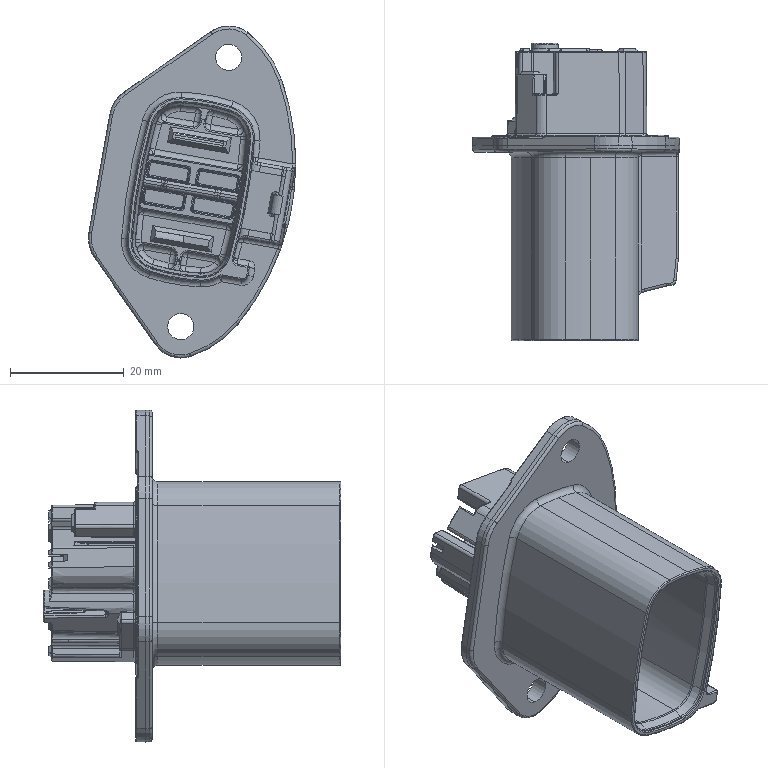Part | SolidWorks | features BaseBody 1 | 1 solid | 1349 faces | box 36.383 x 52.2 x 58.261 mm | volume 12719 mm3 | cylinder 463 | plane 357 | spline 276 | torus 159 | sphere 52 | cone 42 | commonest cylinder face diameters 0.4 x154 1 x73 0.6 x67 0.2 x49 2 x37 0.5 x22